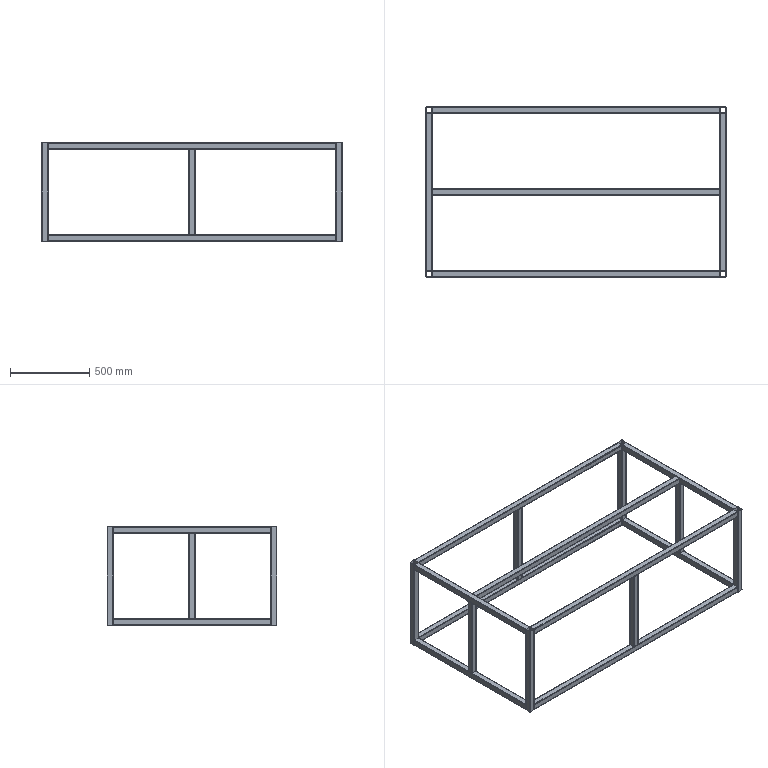Part | SolidWorks | features WeldCornerFeat 22, WeldMemberFeat 5, 3DProfileFeature 3, WeldmentFeature 1 | 17 solids | 306 faces | box 1890 x 1070 x 620 mm | volume 5183789 mm3 | plane 170 | cylinder 136 | commonest cylinder face diameters 4 x68 8 x68